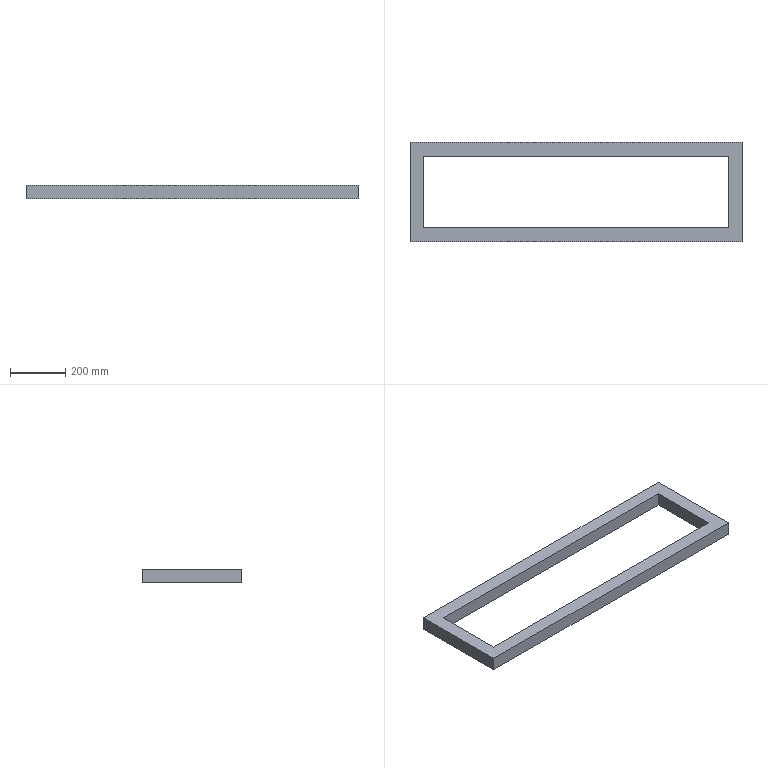Part | STEP file | 1 solid | 10 faces | box 1200 x 359.164 x 50 mm | volume 7295820 mm3 | plane 10
STEP:
#1=CARTESIAN_POINT('',(0.,0.,0.));
#2=DIRECTION('',(0.,0.,1.));
#3=DIRECTION('',(1.,0.,0.));
#4=AXIS2_PLACEMENT_3D('',#1,#2,#3);
#5=CARTESIAN_POINT('',(-550.,-500.,343.641));
#6=VERTEX_POINT('',#5);
#7=CARTESIAN_POINT('',(-550.,-240.836,343.641));
#8=VERTEX_POINT('',#7);
#9=CARTESIAN_POINT('',(-550.,-240.836,343.641));
#10=DIRECTION('',(0.,1.,0.));
#11=VECTOR('',#10,1.);
#12=LINE('',#9,#11);
#13=CARTESIAN_POINT('',(860.,-500.,343.641));
#14=DIRECTION('',(0.,0.,1.));
#15=DIRECTION('',(1.,0.,0.));
#16=AXIS2_PLACEMENT_3D('',#13,#14,#15);
#17=PLANE('',#16);
#18=CARTESIAN_POINT('',(-1410.,259.164));
#19=DIRECTION('',(0.,1.));
#20=VECTOR('',#19,1.);
#21=LINE('',#18,#20);
#22=(GEOMETRIC_REPRESENTATION_CONTEXT(2)PARAMETRIC_REPRESENTATION_CONTEXT()REPRESENTATION_CONTEXT('',''));
#23=DEFINITIONAL_REPRESENTATION('',(#21),#22);
#24=PCURVE('',#17,#23);
#25=CARTESIAN_POINT('',(-550.,-240.836,-806.359));
#26=DIRECTION('',(-1.,0.,0.));
#27=DIRECTION('',(0.,0.,1.));
#28=AXIS2_PLACEMENT_3D('',#25,#26,#27);
#29=PLANE('',#28);
#30=CARTESIAN_POINT('',(1150.,0.));
#31=DIRECTION('',(0.,1.));
#32=VECTOR('',#31,1.);
#33=LINE('',#30,#32);
#34=(GEOMETRIC_REPRESENTATION_CONTEXT(2)PARAMETRIC_REPRESENTATION_CONTEXT()REPRESENTATION_CONTEXT('',''));
#35=DEFINITIONAL_REPRESENTATION('',(#33),#34);
#36=PCURVE('',#29,#35);
#37=SURFACE_CURVE('',#12,(#24,#36),.PCURVE_S1.);
#38=EDGE_CURVE('',#6,#8,#37,.T.);
#39=ORIENTED_EDGE('',*,*,#38,.F.);
#40=CARTESIAN_POINT('',(550.,-500.,343.641));
#41=VERTEX_POINT('',#40);
#42=CARTESIAN_POINT('',(-550.,-500.,343.641));
#43=DIRECTION('',(-1.,0.,0.));
#44=VECTOR('',#43,1.);
#45=LINE('',#42,#44);
#46=CARTESIAN_POINT('',(-1410.,0.));
#47=DIRECTION('',(-1.,0.));
#48=VECTOR('',#47,1.);
#49=LINE('',#46,#48);
#50=(GEOMETRIC_REPRESENTATION_CONTEXT(2)PARAMETRIC_REPRESENTATION_CONTEXT()REPRESENTATION_CONTEXT('',''));
#51=DEFINITIONAL_REPRESENTATION('',(#49),#50);
#52=PCURVE('',#17,#51);
#53=CARTESIAN_POINT('',(-550.,-500.,-806.359));
#54=DIRECTION('',(0.,-1.,0.));
#55=DIRECTION('',(1.,0.,0.));
#56=AXIS2_PLACEMENT_3D('',#53,#54,#55);
#57=PLANE('',#56);
#58=CARTESIAN_POINT('',(0.,1150.));
#59=DIRECTION('',(-1.,0.));
#60=VECTOR('',#59,1.);
#61=LINE('',#58,#60);
#62=(GEOMETRIC_REPRESENTATION_CONTEXT(2)PARAMETRIC_REPRESENTATION_CONTEXT()REPRESENTATION_CONTEXT('',''));
#63=DEFINITIONAL_REPRESENTATION('',(#61),#62);
#64=PCURVE('',#57,#63);
#65=SURFACE_CURVE('',#45,(#52,#64),.PCURVE_S1.);
#66=EDGE_CURVE('',#41,#6,#65,.T.);
#67=ORIENTED_EDGE('',*,*,#66,.F.);
#68=CARTESIAN_POINT('',(550.,-240.836,343.641));
#69=VERTEX_POINT('',#68);
#70=CARTESIAN_POINT('',(550.,-500.,343.641));
#71=DIRECTION('',(0.,-1.,0.));
#72=VECTOR('',#71,1.);
#73=LINE('',#70,#72);
#74=CARTESIAN_POINT('',(-310.,0.));
#75=DIRECTION('',(0.,-1.));
#76=VECTOR('',#75,1.);
#77=LINE('',#74,#76);
#78=(GEOMETRIC_REPRESENTATION_CONTEXT(2)PARAMETRIC_REPRESENTATION_CONTEXT()REPRESENTATION_CONTEXT('',''));
#79=DEFINITIONAL_REPRESENTATION('',(#77),#78);
#80=PCURVE('',#17,#79);
#81=CARTESIAN_POINT('',(550.,-500.,-806.359));
#82=DIRECTION('',(1.,0.,0.));
#83=DIRECTION('',(0.,1.,0.));
#84=AXIS2_PLACEMENT_3D('',#81,#82,#83);
#85=PLANE('',#84);
#86=CARTESIAN_POINT('',(0.,1150.));
#87=DIRECTION('',(-1.,0.));
#88=VECTOR('',#87,1.);
#89=LINE('',#86,#88);
#90=(GEOMETRIC_REPRESENTATION_CONTEXT(2)PARAMETRIC_REPRESENTATION_CONTEXT()REPRESENTATION_CONTEXT('',''));
#91=DEFINITIONAL_REPRESENTATION('',(#89),#90);
#92=PCURVE('',#85,#91);
#93=SURFACE_CURVE('',#73,(#80,#92),.PCURVE_S1.);
#94=EDGE_CURVE('',#69,#41,#93,.T.);
#95=ORIENTED_EDGE('',*,*,#94,.F.);
#96=CARTESIAN_POINT('',(550.,-240.836,343.641));
#97=DIRECTION('',(1.,0.,0.));
#98=VECTOR('',#97,1.);
#99=LINE('',#96,#98);
#100=CARTESIAN_POINT('',(-310.,259.164));
#101=DIRECTION('',(1.,0.));
#102=VECTOR('',#101,1.);
#103=LINE('',#100,#102);
#104=(GEOMETRIC_REPRESENTATION_CONTEXT(2)PARAMETRIC_REPRESENTATION_CONTEXT()REPRESENTATION_CONTEXT('',''));
#105=DEFINITIONAL_REPRESENTATION('',(#103),#104);
#106=PCURVE('',#17,#105);
#107=CARTESIAN_POINT('',(550.,-240.836,-806.359));
#108=DIRECTION('',(0.,1.,0.));
#109=DIRECTION('',(-1.,0.,0.));
#110=AXIS2_PLACEMENT_3D('',#107,#108,#109);
#111=PLANE('',#110);
#112=CARTESIAN_POINT('',(0.,1150.));
#113=DIRECTION('',(-1.,0.));
#114=VECTOR('',#113,1.);
#115=LINE('',#112,#114);
#116=(GEOMETRIC_REPRESENTATION_CONTEXT(2)PARAMETRIC_REPRESENTATION_CONTEXT()REPRESENTATION_CONTEXT('',''));
#117=DEFINITIONAL_REPRESENTATION('',(#115),#116);
#118=PCURVE('',#111,#117);
#119=SURFACE_CURVE('',#99,(#106,#118),.PCURVE_S1.);
#120=EDGE_CURVE('',#8,#69,#119,.T.);
#121=ORIENTED_EDGE('',*,*,#120,.F.);
#122=EDGE_LOOP('',(#39,#67,#95,#121));
#123=FACE_BOUND('',#122,.T.);
#124=CARTESIAN_POINT('',(600.,-190.836,343.641));
#125=VERTEX_POINT('',#124);
#126=CARTESIAN_POINT('',(600.,-550.,343.641));
#127=VERTEX_POINT('',#126);
#128=CARTESIAN_POINT('',(600.,0.,343.641));
#129=DIRECTION('',(0.,-1.,0.));
#130=VECTOR('',#129,1.);
#131=LINE('',#128,#130);
#132=CARTESIAN_POINT('',(-260.,500.));
#133=DIRECTION('',(0.,-1.));
#134=VECTOR('',#133,1.);
#135=LINE('',#132,#134);
#136=(GEOMETRIC_REPRESENTATION_CONTEXT(2)PARAMETRIC_REPRESENTATION_CONTEXT()REPRESENTATION_CONTEXT('',''));
#137=DEFINITIONAL_REPRESENTATION('',(#135),#136);
#138=PCURVE('',#17,#137);
#139=CARTESIAN_POINT('',(600.,0.,203.641));
#140=DIRECTION('',(1.,0.,0.));
#141=DIRECTION('',(0.,1.,0.));
#142=AXIS2_PLACEMENT_3D('',#139,#140,#141);
#143=PLANE('',#142);
#144=CARTESIAN_POINT('',(0.,140.));
#145=DIRECTION('',(-1.,0.));
#146=VECTOR('',#145,1.);
#147=LINE('',#144,#146);
#148=(GEOMETRIC_REPRESENTATION_CONTEXT(2)PARAMETRIC_REPRESENTATION_CONTEXT()REPRESENTATION_CONTEXT('',''));
#149=DEFINITIONAL_REPRESENTATION('',(#147),#148);
#150=PCURVE('',#143,#149);
#151=SURFACE_CURVE('',#131,(#138,#150),.PCURVE_S1.);
#152=EDGE_CURVE('',#125,#127,#151,.T.);
#153=ORIENTED_EDGE('',*,*,#152,.T.);
#154=CARTESIAN_POINT('',(-600.,-550.,343.641));
#155=VERTEX_POINT('',#154);
#156=CARTESIAN_POINT('',(0.,-550.,343.641));
#157=DIRECTION('',(-1.,0.,0.));
#158=VECTOR('',#157,1.);
#159=LINE('',#156,#158);
#160=CARTESIAN_POINT('',(-860.,-50.));
#161=DIRECTION('',(-1.,0.));
#162=VECTOR('',#161,1.);
#163=LINE('',#160,#162);
#164=(GEOMETRIC_REPRESENTATION_CONTEXT(2)PARAMETRIC_REPRESENTATION_CONTEXT()REPRESENTATION_CONTEXT('',''));
#165=DEFINITIONAL_REPRESENTATION('',(#163),#164);
#166=PCURVE('',#17,#165);
#167=CARTESIAN_POINT('',(0.,-550.,203.641));
#168=DIRECTION('',(0.,-1.,0.));
#169=DIRECTION('',(1.,0.,0.));
#170=AXIS2_PLACEMENT_3D('',#167,#168,#169);
#171=PLANE('',#170);
#172=CARTESIAN_POINT('',(0.,140.));
#173=DIRECTION('',(-1.,0.));
#174=VECTOR('',#173,1.);
#175=LINE('',#172,#174);
#176=(GEOMETRIC_REPRESENTATION_CONTEXT(2)PARAMETRIC_REPRESENTATION_CONTEXT()REPRESENTATION_CONTEXT('',''));
#177=DEFINITIONAL_REPRESENTATION('',(#175),#176);
#178=PCURVE('',#171,#177);
#179=SURFACE_CURVE('',#159,(#166,#178),.PCURVE_S1.);
#180=EDGE_CURVE('',#127,#155,#179,.T.);
#181=ORIENTED_EDGE('',*,*,#180,.T.);
#182=CARTESIAN_POINT('',(-600.,-190.836,343.641));
#183=VERTEX_POINT('',#182);
#184=CARTESIAN_POINT('',(-600.,-500.,343.641));
#185=DIRECTION('',(0.,1.,0.));
#186=VECTOR('',#185,1.);
#187=LINE('',#184,#186);
#188=CARTESIAN_POINT('',(-1460.,0.));
#189=DIRECTION('',(0.,1.));
#190=VECTOR('',#189,1.);
#191=LINE('',#188,#190);
#192=(GEOMETRIC_REPRESENTATION_CONTEXT(2)PARAMETRIC_REPRESENTATION_CONTEXT()REPRESENTATION_CONTEXT('',''));
#193=DEFINITIONAL_REPRESENTATION('',(#191),#192);
#194=PCURVE('',#17,#193);
#195=CARTESIAN_POINT('',(-600.,0.,203.641));
#196=DIRECTION('',(1.,0.,0.));
#197=DIRECTION('',(0.,0.,-1.));
#198=AXIS2_PLACEMENT_3D('',#195,#196,#197);
#199=PLANE('',#198);
#200=CARTESIAN_POINT('',(-140.,-500.));
#201=DIRECTION('',(0.,1.));
#202=VECTOR('',#201,1.);
#203=LINE('',#200,#202);
#204=(GEOMETRIC_REPRESENTATION_CONTEXT(2)PARAMETRIC_REPRESENTATION_CONTEXT()REPRESENTATION_CONTEXT('',''));
#205=DEFINITIONAL_REPRESENTATION('',(#203),#204);
#206=PCURVE('',#199,#205);
#207=SURFACE_CURVE('',#187,(#194,#206),.PCURVE_S1.);
#208=EDGE_CURVE('',#155,#183,#207,.T.);
#209=ORIENTED_EDGE('',*,*,#208,.T.);
#210=CARTESIAN_POINT('',(-550.,-190.836,343.641));
#211=DIRECTION('',(1.,0.,0.));
#212=VECTOR('',#211,1.);
#213=LINE('',#210,#212);
#214=CARTESIAN_POINT('',(-1410.,309.164));
#215=DIRECTION('',(1.,0.));
#216=VECTOR('',#215,1.);
#217=LINE('',#214,#216);
#218=(GEOMETRIC_REPRESENTATION_CONTEXT(2)PARAMETRIC_REPRESENTATION_CONTEXT()REPRESENTATION_CONTEXT('',''));
#219=DEFINITIONAL_REPRESENTATION('',(#217),#218);
#220=PCURVE('',#17,#219);
#221=CARTESIAN_POINT('',(-600.,-190.836,203.641));
#222=DIRECTION('',(0.,1.,0.));
#223=DIRECTION('',(-1.,0.,0.));
#224=AXIS2_PLACEMENT_3D('',#221,#222,#223);
#225=PLANE('',#224);
#226=CARTESIAN_POINT('',(-50.,140.));
#227=DIRECTION('',(-1.,0.));
#228=VECTOR('',#227,1.);
#229=LINE('',#226,#228);
#230=(GEOMETRIC_REPRESENTATION_CONTEXT(2)PARAMETRIC_REPRESENTATION_CONTEXT()REPRESENTATION_CONTEXT('',''));
#231=DEFINITIONAL_REPRESENTATION('',(#229),#230);
#232=PCURVE('',#225,#231);
#233=SURFACE_CURVE('',#213,(#220,#232),.PCURVE_S1.);
#234=EDGE_CURVE('',#183,#125,#233,.T.);
#235=ORIENTED_EDGE('',*,*,#234,.T.);
#236=EDGE_LOOP('',(#153,#181,#209,#235));
#237=FACE_BOUND('',#236,.T.);
#238=ADVANCED_FACE('',(#123,#237),#17,.F.);
#239=CARTESIAN_POINT('',(-600.,-550.,393.641));
#240=VERTEX_POINT('',#239);
#241=CARTESIAN_POINT('',(-600.,-550.,203.641));
#242=DIRECTION('',(0.,0.,-1.));
#243=VECTOR('',#242,1.);
#244=LINE('',#241,#243);
#245=CARTESIAN_POINT('',(-600.,0.));
#246=DIRECTION('',(0.,-1.));
#247=VECTOR('',#246,1.);
#248=LINE('',#245,#247);
#249=(GEOMETRIC_REPRESENTATION_CONTEXT(2)PARAMETRIC_REPRESENTATION_CONTEXT()REPRESENTATION_CONTEXT('',''));
#250=DEFINITIONAL_REPRESENTATION('',(#248),#249);
#251=PCURVE('',#171,#250);
#252=CARTESIAN_POINT('',(0.,-550.));
#253=DIRECTION('',(1.,0.));
#254=VECTOR('',#253,1.);
#255=LINE('',#252,#254);
#256=(GEOMETRIC_REPRESENTATION_CONTEXT(2)PARAMETRIC_REPRESENTATION_CONTEXT()REPRESENTATION_CONTEXT('',''));
#257=DEFINITIONAL_REPRESENTATION('',(#255),#256);
#258=PCURVE('',#199,#257);
#259=SURFACE_CURVE('',#244,(#251,#258),.PCURVE_S1.);
#260=EDGE_CURVE('',#240,#155,#259,.T.);
#261=ORIENTED_EDGE('',*,*,#260,.T.);
#262=ORIENTED_EDGE('',*,*,#180,.F.);
#263=CARTESIAN_POINT('',(600.,-550.,393.641));
#264=VERTEX_POINT('',#263);
#265=CARTESIAN_POINT('',(600.,-550.,203.641));
#266=DIRECTION('',(0.,0.,-1.));
#267=VECTOR('',#266,1.);
#268=LINE('',#265,#267);
#269=CARTESIAN_POINT('',(600.,0.));
#270=DIRECTION('',(0.,-1.));
#271=VECTOR('',#270,1.);
#272=LINE('',#269,#271);
#273=(GEOMETRIC_REPRESENTATION_CONTEXT(2)PARAMETRIC_REPRESENTATION_CONTEXT()REPRESENTATION_CONTEXT('',''));
#274=DEFINITIONAL_REPRESENTATION('',(#272),#273);
#275=PCURVE('',#171,#274);
#276=CARTESIAN_POINT('',(-550.,0.));
#277=DIRECTION('',(0.,-1.));
#278=VECTOR('',#277,1.);
#279=LINE('',#276,#278);
#280=(GEOMETRIC_REPRESENTATION_CONTEXT(2)PARAMETRIC_REPRESENTATION_CONTEXT()REPRESENTATION_CONTEXT('',''));
#281=DEFINITIONAL_REPRESENTATION('',(#279),#280);
#282=PCURVE('',#143,#281);
#283=SURFACE_CURVE('',#268,(#275,#282),.PCURVE_S1.);
#284=EDGE_CURVE('',#264,#127,#283,.T.);
#285=ORIENTED_EDGE('',*,*,#284,.F.);
#286=CARTESIAN_POINT('',(600.,-550.,393.641));
#287=DIRECTION('',(1.,0.,0.));
#288=VECTOR('',#287,1.);
#289=LINE('',#286,#288);
#290=CARTESIAN_POINT('',(600.,190.));
#291=DIRECTION('',(1.,0.));
#292=VECTOR('',#291,1.);
#293=LINE('',#290,#292);
#294=(GEOMETRIC_REPRESENTATION_CONTEXT(2)PARAMETRIC_REPRESENTATION_CONTEXT()REPRESENTATION_CONTEXT('',''));
#295=DEFINITIONAL_REPRESENTATION('',(#293),#294);
#296=PCURVE('',#171,#295);
#297=CARTESIAN_POINT('',(0.,0.,393.641));
#298=DIRECTION('',(0.,0.,-1.));
#299=DIRECTION('',(-1.,0.,0.));
#300=AXIS2_PLACEMENT_3D('',#297,#298,#299);
#301=PLANE('',#300);
#302=CARTESIAN_POINT('',(-600.,-550.));
#303=DIRECTION('',(-1.,0.));
#304=VECTOR('',#303,1.);
#305=LINE('',#302,#304);
#306=(GEOMETRIC_REPRESENTATION_CONTEXT(2)PARAMETRIC_REPRESENTATION_CONTEXT()REPRESENTATION_CONTEXT('',''));
#307=DEFINITIONAL_REPRESENTATION('',(#305),#306);
#308=PCURVE('',#301,#307);
#309=SURFACE_CURVE('',#289,(#296,#308),.PCURVE_S1.);
#310=EDGE_CURVE('',#240,#264,#309,.T.);
#311=ORIENTED_EDGE('',*,*,#310,.F.);
#312=EDGE_LOOP('',(#261,#262,#285,#311));
#313=FACE_BOUND('',#312,.T.);
#314=ADVANCED_FACE('',(#313),#171,.T.);
#315=CARTESIAN_POINT('',(550.,-500.,393.641));
#316=VERTEX_POINT('',#315);
#317=CARTESIAN_POINT('',(550.,-500.,-806.359));
#318=DIRECTION('',(0.,0.,1.));
#319=VECTOR('',#318,1.);
#320=LINE('',#317,#319);
#321=CARTESIAN_POINT('',(1100.,0.));
#322=DIRECTION('',(0.,1.));
#323=VECTOR('',#322,1.);
#324=LINE('',#321,#323);
#325=(GEOMETRIC_REPRESENTATION_CONTEXT(2)PARAMETRIC_REPRESENTATION_CONTEXT()REPRESENTATION_CONTEXT('',''));
#326=DEFINITIONAL_REPRESENTATION('',(#324),#325);
#327=PCURVE('',#57,#326);
#328=CARTESIAN_POINT('',(0.,0.));
#329=DIRECTION('',(0.,1.));
#330=VECTOR('',#329,1.);
#331=LINE('',#328,#330);
#332=(GEOMETRIC_REPRESENTATION_CONTEXT(2)PARAMETRIC_REPRESENTATION_CONTEXT()REPRESENTATION_CONTEXT('',''));
#333=DEFINITIONAL_REPRESENTATION('',(#331),#332);
#334=PCURVE('',#85,#333);
#335=SURFACE_CURVE('',#320,(#327,#334),.PCURVE_S1.);
#336=EDGE_CURVE('',#41,#316,#335,.T.);
#337=ORIENTED_EDGE('',*,*,#336,.F.);
#338=ORIENTED_EDGE('',*,*,#66,.T.);
#339=CARTESIAN_POINT('',(-550.,-500.,393.641));
#340=VERTEX_POINT('',#339);
#341=CARTESIAN_POINT('',(-550.,-500.,-806.359));
#342=DIRECTION('',(0.,0.,1.));
#343=VECTOR('',#342,1.);
#344=LINE('',#341,#343);
#345=CARTESIAN_POINT('',(0.,0.));
#346=DIRECTION('',(0.,1.));
#347=VECTOR('',#346,1.);
#348=LINE('',#345,#347);
#349=(GEOMETRIC_REPRESENTATION_CONTEXT(2)PARAMETRIC_REPRESENTATION_CONTEXT()REPRESENTATION_CONTEXT('',''));
#350=DEFINITIONAL_REPRESENTATION('',(#348),#349);
#351=PCURVE('',#57,#350);
#352=CARTESIAN_POINT('',(0.,-259.164));
#353=DIRECTION('',(1.,0.));
#354=VECTOR('',#353,1.);
#355=LINE('',#352,#354);
#356=(GEOMETRIC_REPRESENTATION_CONTEXT(2)PARAMETRIC_REPRESENTATION_CONTEXT()REPRESENTATION_CONTEXT('',''));
#357=DEFINITIONAL_REPRESENTATION('',(#355),#356);
#358=PCURVE('',#29,#357);
#359=SURFACE_CURVE('',#344,(#351,#358),.PCURVE_S1.);
#360=EDGE_CURVE('',#6,#340,#359,.T.);
#361=ORIENTED_EDGE('',*,*,#360,.T.);
#362=CARTESIAN_POINT('',(-550.,-500.,393.641));
#363=DIRECTION('',(1.,0.,0.));
#364=VECTOR('',#363,1.);
#365=LINE('',#362,#364);
#366=CARTESIAN_POINT('',(0.,1200.));
#367=DIRECTION('',(1.,0.));
#368=VECTOR('',#367,1.);
#369=LINE('',#366,#368);
#370=(GEOMETRIC_REPRESENTATION_CONTEXT(2)PARAMETRIC_REPRESENTATION_CONTEXT()REPRESENTATION_CONTEXT('',''));
#371=DEFINITIONAL_REPRESENTATION('',(#369),#370);
#372=PCURVE('',#57,#371);
#373=CARTESIAN_POINT('',(550.,-500.));
#374=DIRECTION('',(-1.,0.));
#375=VECTOR('',#374,1.);
#376=LINE('',#373,#375);
#377=(GEOMETRIC_REPRESENTATION_CONTEXT(2)PARAMETRIC_REPRESENTATION_CONTEXT()REPRESENTATION_CONTEXT('',''));
#378=DEFINITIONAL_REPRESENTATION('',(#376),#377);
#379=PCURVE('',#301,#378);
#380=SURFACE_CURVE('',#365,(#372,#379),.PCURVE_S1.);
#381=EDGE_CURVE('',#340,#316,#380,.T.);
#382=ORIENTED_EDGE('',*,*,#381,.T.);
#383=EDGE_LOOP('',(#337,#338,#361,#382));
#384=FACE_BOUND('',#383,.T.);
#385=ADVANCED_FACE('',(#384),#57,.F.);
#386=CARTESIAN_POINT('',(600.,-190.836,393.641));
#387=VERTEX_POINT('',#386);
#388=CARTESIAN_POINT('',(600.,-190.836,393.641));
#389=DIRECTION('',(0.,0.,-1.));
#390=VECTOR('',#389,1.);
#391=LINE('',#388,#390);
#392=CARTESIAN_POINT('',(-1200.,190.));
#393=DIRECTION('',(0.,-1.));
#394=VECTOR('',#393,1.);
#395=LINE('',#392,#394);
#396=(GEOMETRIC_REPRESENTATION_CONTEXT(2)PARAMETRIC_REPRESENTATION_CONTEXT()REPRESENTATION_CONTEXT('',''));
#397=DEFINITIONAL_REPRESENTATION('',(#395),#396);
#398=PCURVE('',#225,#397);
#399=CARTESIAN_POINT('',(-190.836,190.));
#400=DIRECTION('',(0.,-1.));
#401=VECTOR('',#400,1.);
#402=LINE('',#399,#401);
#403=(GEOMETRIC_REPRESENTATION_CONTEXT(2)PARAMETRIC_REPRESENTATION_CONTEXT()REPRESENTATION_CONTEXT('',''));
#404=DEFINITIONAL_REPRESENTATION('',(#402),#403);
#405=PCURVE('',#143,#404);
#406=SURFACE_CURVE('',#391,(#398,#405),.PCURVE_S1.);
#407=EDGE_CURVE('',#387,#125,#406,.T.);
#408=ORIENTED_EDGE('',*,*,#407,.T.);
#409=ORIENTED_EDGE('',*,*,#234,.F.);
#410=CARTESIAN_POINT('',(-600.,-190.836,393.641));
#411=VERTEX_POINT('',#410);
#412=CARTESIAN_POINT('',(-600.,-190.836,393.641));
#413=DIRECTION('',(0.,0.,-1.));
#414=VECTOR('',#413,1.);
#415=LINE('',#412,#414);
#416=CARTESIAN_POINT('',(0.,190.));
#417=DIRECTION('',(0.,-1.));
#418=VECTOR('',#417,1.);
#419=LINE('',#416,#418);
#420=(GEOMETRIC_REPRESENTATION_CONTEXT(2)PARAMETRIC_REPRESENTATION_CONTEXT()REPRESENTATION_CONTEXT('',''));
#421=DEFINITIONAL_REPRESENTATION('',(#419),#420);
#422=PCURVE('',#225,#421);
#423=CARTESIAN_POINT('',(-190.,-190.836));
#424=DIRECTION('',(1.,0.));
#425=VECTOR('',#424,1.);
#426=LINE('',#423,#425);
#427=(GEOMETRIC_REPRESENTATION_CONTEXT(2)PARAMETRIC_REPRESENTATION_CONTEXT()REPRESENTATION_CONTEXT('',''));
#428=DEFINITIONAL_REPRESENTATION('',(#426),#427);
#429=PCURVE('',#199,#428);
#430=SURFACE_CURVE('',#415,(#422,#429),.PCURVE_S1.);
#431=EDGE_CURVE('',#411,#183,#430,.T.);
#432=ORIENTED_EDGE('',*,*,#431,.F.);
#433=CARTESIAN_POINT('',(600.,-190.836,393.641));
#434=DIRECTION('',(-1.,0.,0.));
#435=VECTOR('',#434,1.);
#436=LINE('',#433,#435);
#437=CARTESIAN_POINT('',(-1200.,190.));
#438=DIRECTION('',(1.,0.));
#439=VECTOR('',#438,1.);
#440=LINE('',#437,#439);
#441=(GEOMETRIC_REPRESENTATION_CONTEXT(2)PARAMETRIC_REPRESENTATION_CONTEXT()REPRESENTATION_CONTEXT('',''));
#442=DEFINITIONAL_REPRESENTATION('',(#440),#441);
#443=PCURVE('',#225,#442);
#444=CARTESIAN_POINT('',(-600.,-190.836));
#445=DIRECTION('',(1.,0.));
#446=VECTOR('',#445,1.);
#447=LINE('',#444,#446);
#448=(GEOMETRIC_REPRESENTATION_CONTEXT(2)PARAMETRIC_REPRESENTATION_CONTEXT()REPRESENTATION_CONTEXT('',''));
#449=DEFINITIONAL_REPRESENTATION('',(#447),#448);
#450=PCURVE('',#301,#449);
#451=SURFACE_CURVE('',#436,(#443,#450),.PCURVE_S1.);
#452=EDGE_CURVE('',#387,#411,#451,.T.);
#453=ORIENTED_EDGE('',*,*,#452,.F.);
#454=EDGE_LOOP('',(#408,#409,#432,#453));
#455=FACE_BOUND('',#454,.T.);
#456=ADVANCED_FACE('',(#455),#225,.T.);
#457=ORIENTED_EDGE('',*,*,#284,.T.);
#458=ORIENTED_EDGE('',*,*,#152,.F.);
#459=ORIENTED_EDGE('',*,*,#407,.F.);
#460=CARTESIAN_POINT('',(600.,-190.836,393.641));
#461=DIRECTION('',(0.,1.,0.));
#462=VECTOR('',#461,1.);
#463=LINE('',#460,#462);
#464=CARTESIAN_POINT('',(-190.836,190.));
#465=DIRECTION('',(1.,0.));
#466=VECTOR('',#465,1.);
#467=LINE('',#464,#466);
#468=(GEOMETRIC_REPRESENTATION_CONTEXT(2)PARAMETRIC_REPRESENTATION_CONTEXT()REPRESENTATION_CONTEXT('',''));
#469=DEFINITIONAL_REPRESENTATION('',(#467),#468);
#470=PCURVE('',#143,#469);
#471=CARTESIAN_POINT('',(-600.,-190.836));
#472=DIRECTION('',(0.,1.));
#473=VECTOR('',#472,1.);
#474=LINE('',#471,#473);
#475=(GEOMETRIC_REPRESENTATION_CONTEXT(2)PARAMETRIC_REPRESENTATION_CONTEXT()REPRESENTATION_CONTEXT('',''));
#476=DEFINITIONAL_REPRESENTATION('',(#474),#475);
#477=PCURVE('',#301,#476);
#478=SURFACE_CURVE('',#463,(#470,#477),.PCURVE_S1.);
#479=EDGE_CURVE('',#264,#387,#478,.T.);
#480=ORIENTED_EDGE('',*,*,#479,.F.);
#481=EDGE_LOOP('',(#457,#458,#459,#480));
#482=FACE_BOUND('',#481,.T.);
#483=ADVANCED_FACE('',(#482),#143,.T.);
#484=ORIENTED_EDGE('',*,*,#208,.F.);
#485=ORIENTED_EDGE('',*,*,#260,.F.);
#486=CARTESIAN_POINT('',(-600.,-190.836,393.641));
#487=DIRECTION('',(0.,-1.,0.));
#488=VECTOR('',#487,1.);
#489=LINE('',#486,#488);
#490=CARTESIAN_POINT('',(-190.,-190.836));
#491=DIRECTION('',(0.,-1.));
#492=VECTOR('',#491,1.);
#493=LINE('',#490,#492);
#494=(GEOMETRIC_REPRESENTATION_CONTEXT(2)PARAMETRIC_REPRESENTATION_CONTEXT()REPRESENTATION_CONTEXT('',''));
#495=DEFINITIONAL_REPRESENTATION('',(#493),#494);
#496=PCURVE('',#199,#495);
#497=CARTESIAN_POINT('',(600.,-190.836));
#498=DIRECTION('',(0.,-1.));
#499=VECTOR('',#498,1.);
#500=LINE('',#497,#499);
#501=(GEOMETRIC_REPRESENTATION_CONTEXT(2)PARAMETRIC_REPRESENTATION_CONTEXT()REPRESENTATION_CONTEXT('',''));
#502=DEFINITIONAL_REPRESENTATION('',(#500),#501);
#503=PCURVE('',#301,#502);
#504=SURFACE_CURVE('',#489,(#496,#503),.PCURVE_S1.);
#505=EDGE_CURVE('',#411,#240,#504,.T.);
#506=ORIENTED_EDGE('',*,*,#505,.F.);
#507=ORIENTED_EDGE('',*,*,#431,.T.);
#508=EDGE_LOOP('',(#484,#485,#506,#507));
#509=FACE_BOUND('',#508,.T.);
#510=ADVANCED_FACE('',(#509),#199,.F.);
#511=CARTESIAN_POINT('',(-550.,-240.836,393.641));
#512=VERTEX_POINT('',#511);
#513=CARTESIAN_POINT('',(-550.,-240.836,-806.359));
#514=DIRECTION('',(0.,0.,1.));
#515=VECTOR('',#514,1.);
#516=LINE('',#513,#515);
#517=CARTESIAN_POINT('',(1100.,0.));
#518=DIRECTION('',(0.,1.));
#519=VECTOR('',#518,1.);
#520=LINE('',#517,#519);
#521=(GEOMETRIC_REPRESENTATION_CONTEXT(2)PARAMETRIC_REPRESENTATION_CONTEXT()REPRESENTATION_CONTEXT('',''));
#522=DEFINITIONAL_REPRESENTATION('',(#520),#521);
#523=PCURVE('',#111,#522);
#524=CARTESIAN_POINT('',(0.,0.));
#525=DIRECTION('',(1.,0.));
#526=VECTOR('',#525,1.);
#527=LINE('',#524,#526);
#528=(GEOMETRIC_REPRESENTATION_CONTEXT(2)PARAMETRIC_REPRESENTATION_CONTEXT()REPRESENTATION_CONTEXT('',''));
#529=DEFINITIONAL_REPRESENTATION('',(#527),#528);
#530=PCURVE('',#29,#529);
#531=SURFACE_CURVE('',#516,(#523,#530),.PCURVE_S1.);
#532=EDGE_CURVE('',#8,#512,#531,.T.);
#533=ORIENTED_EDGE('',*,*,#532,.F.);
#534=ORIENTED_EDGE('',*,*,#120,.T.);
#535=CARTESIAN_POINT('',(550.,-240.836,393.641));
#536=VERTEX_POINT('',#535);
#537=CARTESIAN_POINT('',(550.,-240.836,-806.359));
#538=DIRECTION('',(0.,0.,1.));
#539=VECTOR('',#538,1.);
#540=LINE('',#537,#539);
#541=CARTESIAN_POINT('',(0.,0.));
#542=DIRECTION('',(0.,1.));
#543=VECTOR('',#542,1.);
#544=LINE('',#541,#543);
#545=(GEOMETRIC_REPRESENTATION_CONTEXT(2)PARAMETRIC_REPRESENTATION_CONTEXT()REPRESENTATION_CONTEXT('',''));
#546=DEFINITIONAL_REPRESENTATION('',(#544),#545);
#547=PCURVE('',#111,#546);
#548=CARTESIAN_POINT('',(259.164,0.));
#549=DIRECTION('',(0.,1.));
#550=VECTOR('',#549,1.);
#551=LINE('',#548,#550);
#552=(GEOMETRIC_REPRESENTATION_CONTEXT(2)PARAMETRIC_REPRESENTATION_CONTEXT()REPRESENTATION_CONTEXT('',''));
#553=DEFINITIONAL_REPRESENTATION('',(#551),#552);
#554=PCURVE('',#85,#553);
#555=SURFACE_CURVE('',#540,(#547,#554),.PCURVE_S1.);
#556=EDGE_CURVE('',#69,#536,#555,.T.);
#557=ORIENTED_EDGE('',*,*,#556,.T.);
#558=CARTESIAN_POINT('',(550.,-240.836,393.641));
#559=DIRECTION('',(-1.,0.,0.));
#560=VECTOR('',#559,1.);
#561=LINE('',#558,#560);
#562=CARTESIAN_POINT('',(0.,1200.));
#563=DIRECTION('',(1.,0.));
#564=VECTOR('',#563,1.);
#565=LINE('',#562,#564);
#566=(GEOMETRIC_REPRESENTATION_CONTEXT(2)PARAMETRIC_REPRESENTATION_CONTEXT()REPRESENTATION_CONTEXT('',''));
#567=DEFINITIONAL_REPRESENTATION('',(#565),#566);
#568=PCURVE('',#111,#567);
#569=CARTESIAN_POINT('',(-550.,-240.836));
#570=DIRECTION('',(1.,0.));
#571=VECTOR('',#570,1.);
#572=LINE('',#569,#571);
#573=(GEOMETRIC_REPRESENTATION_CONTEXT(2)PARAMETRIC_REPRESENTATION_CONTEXT()REPRESENTATION_CONTEXT('',''));
#574=DEFINITIONAL_REPRESENTATION('',(#572),#573);
#575=PCURVE('',#301,#574);
#576=SURFACE_CURVE('',#561,(#568,#575),.PCURVE_S1.);
#577=EDGE_CURVE('',#536,#512,#576,.T.);
#578=ORIENTED_EDGE('',*,*,#577,.T.);
#579=EDGE_LOOP('',(#533,#534,#557,#578));
#580=FACE_BOUND('',#579,.T.);
#581=ADVANCED_FACE('',(#580),#111,.F.);
#582=ORIENTED_EDGE('',*,*,#360,.F.);
#583=ORIENTED_EDGE('',*,*,#38,.T.);
#584=ORIENTED_EDGE('',*,*,#532,.T.);
#585=CARTESIAN_POINT('',(-550.,-240.836,393.641));
#586=DIRECTION('',(0.,-1.,0.));
#587=VECTOR('',#586,1.);
#588=LINE('',#585,#587);
#589=CARTESIAN_POINT('',(1200.,0.));
#590=DIRECTION('',(0.,-1.));
#591=VECTOR('',#590,1.);
#592=LINE('',#589,#591);
#593=(GEOMETRIC_REPRESENTATION_CONTEXT(2)PARAMETRIC_REPRESENTATION_CONTEXT()REPRESENTATION_CONTEXT('',''));
#594=DEFINITIONAL_REPRESENTATION('',(#592),#593);
#595=PCURVE('',#29,#594);
#596=CARTESIAN_POINT('',(550.,-240.836));
#597=DIRECTION('',(0.,-1.));
#598=VECTOR('',#597,1.);
#599=LINE('',#596,#598);
#600=(GEOMETRIC_REPRESENTATION_CONTEXT(2)PARAMETRIC_REPRESENTATION_CONTEXT()REPRESENTATION_CONTEXT('',''));
#601=DEFINITIONAL_REPRESENTATION('',(#599),#600);
#602=PCURVE('',#301,#601);
#603=SURFACE_CURVE('',#588,(#595,#602),.PCURVE_S1.);
#604=EDGE_CURVE('',#512,#340,#603,.T.);
#605=ORIENTED_EDGE('',*,*,#604,.T.);
#606=EDGE_LOOP('',(#582,#583,#584,#605));
#607=FACE_BOUND('',#606,.T.);
#608=ADVANCED_FACE('',(#607),#29,.F.);
#609=ORIENTED_EDGE('',*,*,#556,.F.);
#610=ORIENTED_EDGE('',*,*,#94,.T.);
#611=ORIENTED_EDGE('',*,*,#336,.T.);
#612=CARTESIAN_POINT('',(550.,-500.,393.641));
#613=DIRECTION('',(0.,1.,0.));
#614=VECTOR('',#613,1.);
#615=LINE('',#612,#614);
#616=CARTESIAN_POINT('',(0.,1200.));
#617=DIRECTION('',(1.,0.));
#618=VECTOR('',#617,1.);
#619=LINE('',#616,#618);
#620=(GEOMETRIC_REPRESENTATION_CONTEXT(2)PARAMETRIC_REPRESENTATION_CONTEXT()REPRESENTATION_CONTEXT('',''));
#621=DEFINITIONAL_REPRESENTATION('',(#619),#620);
#622=PCURVE('',#85,#621);
#623=CARTESIAN_POINT('',(-550.,-500.));
#624=DIRECTION('',(0.,1.));
#625=VECTOR('',#624,1.);
#626=LINE('',#623,#625);
#627=(GEOMETRIC_REPRESENTATION_CONTEXT(2)PARAMETRIC_REPRESENTATION_CONTEXT()REPRESENTATION_CONTEXT('',''));
#628=DEFINITIONAL_REPRESENTATION('',(#626),#627);
#629=PCURVE('',#301,#628);
#630=SURFACE_CURVE('',#615,(#622,#629),.PCURVE_S1.);
#631=EDGE_CURVE('',#316,#536,#630,.T.);
#632=ORIENTED_EDGE('',*,*,#631,.T.);
#633=EDGE_LOOP('',(#609,#610,#611,#632));
#634=FACE_BOUND('',#633,.T.);
#635=ADVANCED_FACE('',(#634),#85,.F.);
#636=ORIENTED_EDGE('',*,*,#604,.F.);
#637=ORIENTED_EDGE('',*,*,#577,.F.);
#638=ORIENTED_EDGE('',*,*,#631,.F.);
#639=ORIENTED_EDGE('',*,*,#381,.F.);
#640=EDGE_LOOP('',(#636,#637,#638,#639));
#641=FACE_BOUND('',#640,.T.);
#642=ORIENTED_EDGE('',*,*,#505,.T.);
#643=ORIENTED_EDGE('',*,*,#310,.T.);
#644=ORIENTED_EDGE('',*,*,#479,.T.);
#645=ORIENTED_EDGE('',*,*,#452,.T.);
#646=EDGE_LOOP('',(#642,#643,#644,#645));
#647=FACE_BOUND('',#646,.T.);
#648=ADVANCED_FACE('',(#641,#647),#301,.F.);
#649=CLOSED_SHELL('',(#238,#314,#385,#456,#483,#510,#581,#608,#635,#648));
#650=MANIFOLD_SOLID_BREP('',#649);
#651=(LENGTH_UNIT()NAMED_UNIT(*)SI_UNIT(.MILLI.,.METRE.));
#652=UNCERTAINTY_MEASURE_WITH_UNIT(LENGTH_MEASURE(0.0000001),#651,'','');
#653=(NAMED_UNIT(*)PLANE_ANGLE_UNIT()SI_UNIT($,.RADIAN.));
#654=(NAMED_UNIT(*)SI_UNIT($,.STERADIAN.)SOLID_ANGLE_UNIT());
#655=(GEOMETRIC_REPRESENTATION_CONTEXT(3)GLOBAL_UNCERTAINTY_ASSIGNED_CONTEXT((#652))GLOBAL_UNIT_ASSIGNED_CONTEXT((#651,#653,#654))REPRESENTATION_CONTEXT('',''));
#656=ADVANCED_BREP_SHAPE_REPRESENTATION('',(#4,#650),#655);